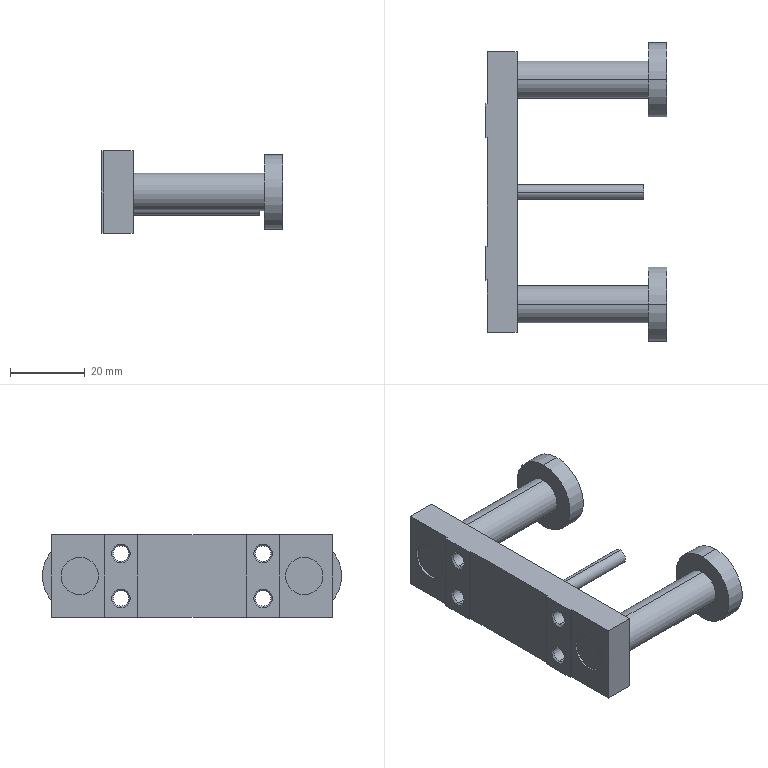Part | STEP file | 2-10 | 1 solid | 59 faces | box 48.5 x 80 x 22 mm | volume 21918 mm3 | cylinder 22 | plane 21 | cone 16 | commonest cylinder face diameters 4.134 x8 10 x8 20 x4 4 x2